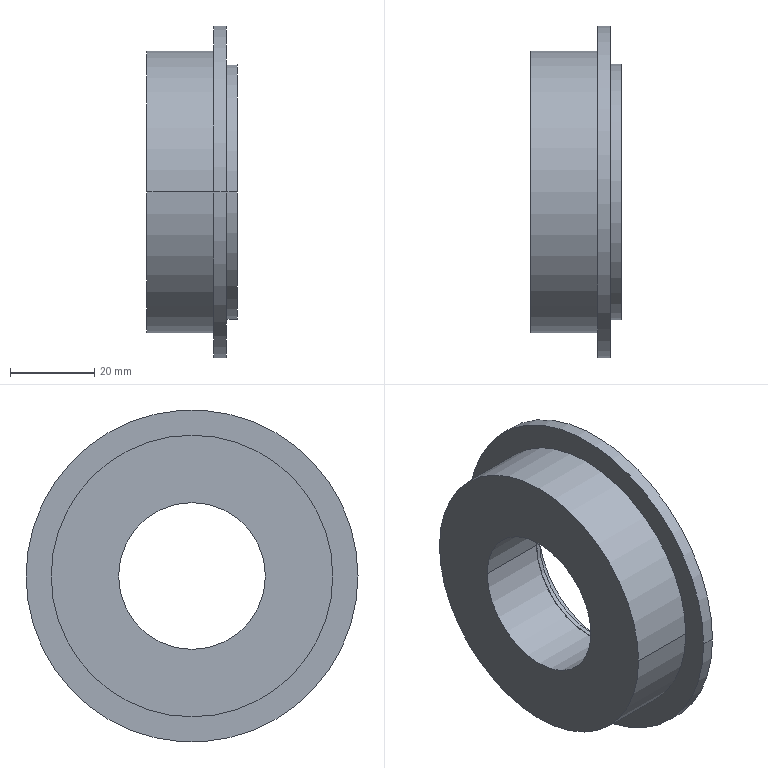Part | SolidWorks | features Revolution 1 | 4 solids | 39 faces | box 21.418 x 78.909 x 78.909 mm | volume 50880 mm3 | cylinder 26 | plane 13 | commonest cylinder face diameters 34.909 x4 40.909 x2 40.984 x2 42.979 x2 44.398 x2 50.004 x2
STEP:
#1=CARTESIAN_POINT('',(77.,20.455,0.));
#2=VERTEX_POINT('',#1);
#3=CARTESIAN_POINT('',(77.,-20.455,0.));
#4=VERTEX_POINT('',#3);
#5=CARTESIAN_POINT('',(77.,0.,0.));
#6=DIRECTION('',(1.,0.,0.));
#7=DIRECTION('',(0.,1.,0.));
#8=AXIS2_PLACEMENT_3D('',#5,#6,#7);
#9=CIRCLE('',#8,20.455);
#10=EDGE_CURVE('',#2,#4,#9,.T.);
#11=ORIENTED_EDGE('',*,*,#10,.T.);
#12=CARTESIAN_POINT('',(90.724,-20.455,0.));
#13=VERTEX_POINT('',#12);
#14=CARTESIAN_POINT('',(0.,-20.455,0.));
#15=DIRECTION('',(1.,0.,0.));
#16=VECTOR('',#15,1000.);
#17=LINE('',#14,#16);
#18=EDGE_CURVE('',#4,#13,#17,.T.);
#19=ORIENTED_EDGE('',*,*,#18,.T.);
#20=CARTESIAN_POINT('',(90.724,20.455,0.));
#21=VERTEX_POINT('',#20);
#22=CARTESIAN_POINT('',(90.724,0.,0.));
#23=DIRECTION('',(1.,0.,0.));
#24=DIRECTION('',(0.,1.,0.));
#25=AXIS2_PLACEMENT_3D('',#22,#23,#24);
#26=CIRCLE('',#25,20.455);
#27=EDGE_CURVE('',#21,#13,#26,.T.);
#28=ORIENTED_EDGE('',*,*,#27,.F.);
#29=CARTESIAN_POINT('',(0.,20.455,0.));
#30=DIRECTION('',(1.,0.,0.));
#31=VECTOR('',#30,1000.);
#32=LINE('',#29,#31);
#33=EDGE_CURVE('',#2,#21,#32,.T.);
#34=ORIENTED_EDGE('',*,*,#33,.F.);
#35=EDGE_LOOP('',(#11,#19,#28,#34));
#36=FACE_OUTER_BOUND('',#35,.T.);
#37=CARTESIAN_POINT('',(0.,0.,0.));
#38=DIRECTION('',(1.,0.,0.));
#39=DIRECTION('',(0.,1.,0.));
#40=AXIS2_PLACEMENT_3D('',#37,#38,#39);
#41=CYLINDRICAL_SURFACE('',#40,20.455);
#42=ADVANCED_FACE('',(#36),#41,.T.);
#43=CARTESIAN_POINT('',(74.143,-17.455,0.));
#44=VERTEX_POINT('',#43);
#45=CARTESIAN_POINT('',(74.143,17.455,0.));
#46=VERTEX_POINT('',#45);
#47=CARTESIAN_POINT('',(74.143,0.,0.));
#48=DIRECTION('',(1.,0.,0.));
#49=DIRECTION('',(0.,1.,0.));
#50=AXIS2_PLACEMENT_3D('',#47,#48,#49);
#51=CIRCLE('',#50,17.455);
#52=EDGE_CURVE('',#44,#46,#51,.T.);
#53=ORIENTED_EDGE('',*,*,#52,.F.);
#54=CARTESIAN_POINT('',(90.724,-17.455,0.));
#55=VERTEX_POINT('',#54);
#56=CARTESIAN_POINT('',(0.,-17.455,0.));
#57=DIRECTION('',(1.,0.,0.));
#58=VECTOR('',#57,1000.);
#59=LINE('',#56,#58);
#60=EDGE_CURVE('',#44,#55,#59,.T.);
#61=ORIENTED_EDGE('',*,*,#60,.T.);
#62=CARTESIAN_POINT('',(90.724,17.455,0.));
#63=VERTEX_POINT('',#62);
#64=CARTESIAN_POINT('',(90.724,0.,0.));
#65=DIRECTION('',(1.,0.,0.));
#66=DIRECTION('',(0.,1.,0.));
#67=AXIS2_PLACEMENT_3D('',#64,#65,#66);
#68=CIRCLE('',#67,17.455);
#69=EDGE_CURVE('',#55,#63,#68,.T.);
#70=ORIENTED_EDGE('',*,*,#69,.T.);
#71=CARTESIAN_POINT('',(0.,17.455,0.));
#72=DIRECTION('',(1.,0.,0.));
#73=VECTOR('',#72,1000.);
#74=LINE('',#71,#73);
#75=EDGE_CURVE('',#46,#63,#74,.T.);
#76=ORIENTED_EDGE('',*,*,#75,.F.);
#77=EDGE_LOOP('',(#53,#61,#70,#76));
#78=FACE_OUTER_BOUND('',#77,.T.);
#79=CARTESIAN_POINT('',(0.,0.,0.));
#80=DIRECTION('',(1.,0.,0.));
#81=DIRECTION('',(0.,1.,0.));
#82=AXIS2_PLACEMENT_3D('',#79,#80,#81);
#83=CYLINDRICAL_SURFACE('',#82,17.455);
#84=ADVANCED_FACE('',(#78),#83,.F.);
#85=CARTESIAN_POINT('',(74.143,33.455,0.));
#86=VERTEX_POINT('',#85);
#87=CARTESIAN_POINT('',(74.143,-33.455,0.));
#88=VERTEX_POINT('',#87);
#89=CARTESIAN_POINT('',(74.143,0.,0.));
#90=DIRECTION('',(1.,0.,0.));
#91=DIRECTION('',(0.,1.,0.));
#92=AXIS2_PLACEMENT_3D('',#89,#90,#91);
#93=CIRCLE('',#92,33.455);
#94=EDGE_CURVE('',#86,#88,#93,.T.);
#95=ORIENTED_EDGE('',*,*,#94,.T.);
#96=CARTESIAN_POINT('',(90.,-33.455,0.));
#97=VERTEX_POINT('',#96);
#98=CARTESIAN_POINT('',(0.,-33.455,0.));
#99=DIRECTION('',(1.,0.,0.));
#100=VECTOR('',#99,1000.);
#101=LINE('',#98,#100);
#102=EDGE_CURVE('',#88,#97,#101,.T.);
#103=ORIENTED_EDGE('',*,*,#102,.T.);
#104=CARTESIAN_POINT('',(90.,33.455,0.));
#105=VERTEX_POINT('',#104);
#106=CARTESIAN_POINT('',(90.,0.,0.));
#107=DIRECTION('',(1.,0.,0.));
#108=DIRECTION('',(0.,1.,0.));
#109=AXIS2_PLACEMENT_3D('',#106,#107,#108);
#110=CIRCLE('',#109,33.455);
#111=EDGE_CURVE('',#105,#97,#110,.T.);
#112=ORIENTED_EDGE('',*,*,#111,.F.);
#113=CARTESIAN_POINT('',(0.,33.455,0.));
#114=DIRECTION('',(1.,0.,0.));
#115=VECTOR('',#114,1000.);
#116=LINE('',#113,#115);
#117=EDGE_CURVE('',#86,#105,#116,.T.);
#118=ORIENTED_EDGE('',*,*,#117,.F.);
#119=EDGE_LOOP('',(#95,#103,#112,#118));
#120=FACE_OUTER_BOUND('',#119,.T.);
#121=CARTESIAN_POINT('',(0.,0.,0.));
#122=DIRECTION('',(1.,0.,0.));
#123=DIRECTION('',(0.,1.,0.));
#124=AXIS2_PLACEMENT_3D('',#121,#122,#123);
#125=CYLINDRICAL_SURFACE('',#124,33.455);
#126=ADVANCED_FACE('',(#120),#125,.T.);
#127=CARTESIAN_POINT('',(90.,39.455,0.));
#128=VERTEX_POINT('',#127);
#129=CARTESIAN_POINT('',(90.,-39.455,0.));
#130=VERTEX_POINT('',#129);
#131=CARTESIAN_POINT('',(90.,0.,0.));
#132=DIRECTION('',(1.,0.,0.));
#133=DIRECTION('',(0.,1.,0.));
#134=AXIS2_PLACEMENT_3D('',#131,#132,#133);
#135=CIRCLE('',#134,39.455);
#136=EDGE_CURVE('',#128,#130,#135,.T.);
#137=ORIENTED_EDGE('',*,*,#136,.T.);
#138=CARTESIAN_POINT('',(93.,-39.455,0.));
#139=VERTEX_POINT('',#138);
#140=CARTESIAN_POINT('',(0.,-39.455,0.));
#141=DIRECTION('',(1.,0.,0.));
#142=VECTOR('',#141,1000.);
#143=LINE('',#140,#142);
#144=EDGE_CURVE('',#130,#139,#143,.T.);
#145=ORIENTED_EDGE('',*,*,#144,.T.);
#146=CARTESIAN_POINT('',(93.,39.455,0.));
#147=VERTEX_POINT('',#146);
#148=CARTESIAN_POINT('',(93.,0.,0.));
#149=DIRECTION('',(1.,0.,0.));
#150=DIRECTION('',(0.,1.,0.));
#151=AXIS2_PLACEMENT_3D('',#148,#149,#150);
#152=CIRCLE('',#151,39.455);
#153=EDGE_CURVE('',#147,#139,#152,.T.);
#154=ORIENTED_EDGE('',*,*,#153,.F.);
#155=CARTESIAN_POINT('',(0.,39.455,0.));
#156=DIRECTION('',(1.,0.,0.));
#157=VECTOR('',#156,1000.);
#158=LINE('',#155,#157);
#159=EDGE_CURVE('',#128,#147,#158,.T.);
#160=ORIENTED_EDGE('',*,*,#159,.F.);
#161=EDGE_LOOP('',(#137,#145,#154,#160));
#162=FACE_OUTER_BOUND('',#161,.T.);
#163=CARTESIAN_POINT('',(0.,0.,0.));
#164=DIRECTION('',(1.,0.,0.));
#165=DIRECTION('',(0.,1.,0.));
#166=AXIS2_PLACEMENT_3D('',#163,#164,#165);
#167=CYLINDRICAL_SURFACE('',#166,39.455);
#168=ADVANCED_FACE('',(#162),#167,.T.);
#169=CARTESIAN_POINT('',(77.,-30.955,0.));
#170=VERTEX_POINT('',#169);
#171=CARTESIAN_POINT('',(77.,30.955,0.));
#172=VERTEX_POINT('',#171);
#173=CARTESIAN_POINT('',(77.,0.,0.));
#174=DIRECTION('',(1.,0.,0.));
#175=DIRECTION('',(0.,1.,0.));
#176=AXIS2_PLACEMENT_3D('',#173,#174,#175);
#177=CIRCLE('',#176,30.955);
#178=EDGE_CURVE('',#170,#172,#177,.T.);
#179=ORIENTED_EDGE('',*,*,#178,.F.);
#180=CARTESIAN_POINT('',(93.,-30.955,0.));
#181=VERTEX_POINT('',#180);
#182=CARTESIAN_POINT('',(0.,-30.955,0.));
#183=DIRECTION('',(1.,0.,0.));
#184=VECTOR('',#183,1000.);
#185=LINE('',#182,#184);
#186=EDGE_CURVE('',#170,#181,#185,.T.);
#187=ORIENTED_EDGE('',*,*,#186,.T.);
#188=CARTESIAN_POINT('',(93.,30.955,0.));
#189=VERTEX_POINT('',#188);
#190=CARTESIAN_POINT('',(93.,0.,0.));
#191=DIRECTION('',(1.,0.,0.));
#192=DIRECTION('',(0.,1.,0.));
#193=AXIS2_PLACEMENT_3D('',#190,#191,#192);
#194=CIRCLE('',#193,30.955);
#195=EDGE_CURVE('',#181,#189,#194,.T.);
#196=ORIENTED_EDGE('',*,*,#195,.T.);
#197=CARTESIAN_POINT('',(0.,30.955,0.));
#198=DIRECTION('',(1.,0.,0.));
#199=VECTOR('',#198,1000.);
#200=LINE('',#197,#199);
#201=EDGE_CURVE('',#172,#189,#200,.T.);
#202=ORIENTED_EDGE('',*,*,#201,.F.);
#203=EDGE_LOOP('',(#179,#187,#196,#202));
#204=FACE_OUTER_BOUND('',#203,.T.);
#205=CARTESIAN_POINT('',(0.,0.,0.));
#206=DIRECTION('',(1.,0.,0.));
#207=DIRECTION('',(0.,1.,0.));
#208=AXIS2_PLACEMENT_3D('',#205,#206,#207);
#209=CYLINDRICAL_SURFACE('',#208,30.955);
#210=ADVANCED_FACE('',(#204),#209,.F.);
#211=ORIENTED_EDGE('',*,*,#186,.F.);
#212=CARTESIAN_POINT('',(77.,0.,0.));
#213=DIRECTION('',(1.,0.,0.));
#214=DIRECTION('',(0.,1.,0.));
#215=AXIS2_PLACEMENT_3D('',#212,#213,#214);
#216=CIRCLE('',#215,30.955);
#217=EDGE_CURVE('',#172,#170,#216,.T.);
#218=ORIENTED_EDGE('',*,*,#217,.F.);
#219=ORIENTED_EDGE('',*,*,#201,.T.);
#220=CARTESIAN_POINT('',(93.,0.,0.));
#221=DIRECTION('',(1.,0.,0.));
#222=DIRECTION('',(0.,1.,0.));
#223=AXIS2_PLACEMENT_3D('',#220,#221,#222);
#224=CIRCLE('',#223,30.955);
#225=EDGE_CURVE('',#189,#181,#224,.T.);
#226=ORIENTED_EDGE('',*,*,#225,.T.);
#227=EDGE_LOOP('',(#211,#218,#219,#226));
#228=FACE_OUTER_BOUND('',#227,.T.);
#229=CARTESIAN_POINT('',(0.,0.,0.));
#230=DIRECTION('',(1.,0.,0.));
#231=DIRECTION('',(0.,1.,0.));
#232=AXIS2_PLACEMENT_3D('',#229,#230,#231);
#233=CYLINDRICAL_SURFACE('',#232,30.955);
#234=ADVANCED_FACE('',(#228),#233,.F.);
#235=ORIENTED_EDGE('',*,*,#153,.T.);
#236=CARTESIAN_POINT('',(93.,0.,0.));
#237=DIRECTION('',(1.,0.,0.));
#238=DIRECTION('',(0.,1.,0.));
#239=AXIS2_PLACEMENT_3D('',#236,#237,#238);
#240=CIRCLE('',#239,39.455);
#241=EDGE_CURVE('',#139,#147,#240,.T.);
#242=ORIENTED_EDGE('',*,*,#241,.T.);
#243=EDGE_LOOP('',(#235,#242));
#244=FACE_OUTER_BOUND('',#243,.T.);
#245=ORIENTED_EDGE('',*,*,#225,.F.);
#246=ORIENTED_EDGE('',*,*,#195,.F.);
#247=EDGE_LOOP('',(#245,#246));
#248=FACE_BOUND('',#247,.T.);
#249=CARTESIAN_POINT('',(93.,0.,0.));
#250=DIRECTION('',(1.,0.,0.));
#251=DIRECTION('',(0.,1.,0.));
#252=AXIS2_PLACEMENT_3D('',#249,#250,#251);
#253=PLANE('',#252);
#254=ADVANCED_FACE('',(#244,#248),#253,.T.);
#255=ORIENTED_EDGE('',*,*,#144,.F.);
#256=CARTESIAN_POINT('',(90.,0.,0.));
#257=DIRECTION('',(1.,0.,0.));
#258=DIRECTION('',(0.,1.,0.));
#259=AXIS2_PLACEMENT_3D('',#256,#257,#258);
#260=CIRCLE('',#259,39.455);
#261=EDGE_CURVE('',#130,#128,#260,.T.);
#262=ORIENTED_EDGE('',*,*,#261,.T.);
#263=ORIENTED_EDGE('',*,*,#159,.T.);
#264=ORIENTED_EDGE('',*,*,#241,.F.);
#265=EDGE_LOOP('',(#255,#262,#263,#264));
#266=FACE_OUTER_BOUND('',#265,.T.);
#267=CARTESIAN_POINT('',(0.,0.,0.));
#268=DIRECTION('',(1.,0.,0.));
#269=DIRECTION('',(0.,1.,0.));
#270=AXIS2_PLACEMENT_3D('',#267,#268,#269);
#271=CYLINDRICAL_SURFACE('',#270,39.455);
#272=ADVANCED_FACE('',(#266),#271,.T.);
#273=ORIENTED_EDGE('',*,*,#136,.F.);
#274=ORIENTED_EDGE('',*,*,#261,.F.);
#275=EDGE_LOOP('',(#273,#274));
#276=FACE_OUTER_BOUND('',#275,.T.);
#277=ORIENTED_EDGE('',*,*,#111,.T.);
#278=CARTESIAN_POINT('',(90.,0.,0.));
#279=DIRECTION('',(1.,0.,0.));
#280=DIRECTION('',(0.,1.,0.));
#281=AXIS2_PLACEMENT_3D('',#278,#279,#280);
#282=CIRCLE('',#281,33.455);
#283=EDGE_CURVE('',#97,#105,#282,.T.);
#284=ORIENTED_EDGE('',*,*,#283,.T.);
#285=EDGE_LOOP('',(#277,#284));
#286=FACE_BOUND('',#285,.T.);
#287=CARTESIAN_POINT('',(90.,0.,0.));
#288=DIRECTION('',(1.,0.,0.));
#289=DIRECTION('',(0.,1.,0.));
#290=AXIS2_PLACEMENT_3D('',#287,#288,#289);
#291=PLANE('',#290);
#292=ADVANCED_FACE('',(#276,#286),#291,.F.);
#293=ORIENTED_EDGE('',*,*,#102,.F.);
#294=CARTESIAN_POINT('',(74.143,0.,0.));
#295=DIRECTION('',(1.,0.,0.));
#296=DIRECTION('',(0.,1.,0.));
#297=AXIS2_PLACEMENT_3D('',#294,#295,#296);
#298=CIRCLE('',#297,33.455);
#299=EDGE_CURVE('',#88,#86,#298,.T.);
#300=ORIENTED_EDGE('',*,*,#299,.T.);
#301=ORIENTED_EDGE('',*,*,#117,.T.);
#302=ORIENTED_EDGE('',*,*,#283,.F.);
#303=EDGE_LOOP('',(#293,#300,#301,#302));
#304=FACE_OUTER_BOUND('',#303,.T.);
#305=CARTESIAN_POINT('',(0.,0.,0.));
#306=DIRECTION('',(1.,0.,0.));
#307=DIRECTION('',(0.,1.,0.));
#308=AXIS2_PLACEMENT_3D('',#305,#306,#307);
#309=CYLINDRICAL_SURFACE('',#308,33.455);
#310=ADVANCED_FACE('',(#304),#309,.T.);
#311=CARTESIAN_POINT('',(74.143,0.,0.));
#312=DIRECTION('',(1.,0.,0.));
#313=DIRECTION('',(0.,1.,0.));
#314=AXIS2_PLACEMENT_3D('',#311,#312,#313);
#315=CIRCLE('',#314,17.455);
#316=EDGE_CURVE('',#46,#44,#315,.T.);
#317=ORIENTED_EDGE('',*,*,#316,.T.);
#318=ORIENTED_EDGE('',*,*,#52,.T.);
#319=EDGE_LOOP('',(#317,#318));
#320=FACE_BOUND('',#319,.T.);
#321=ORIENTED_EDGE('',*,*,#94,.F.);
#322=ORIENTED_EDGE('',*,*,#299,.F.);
#323=EDGE_LOOP('',(#321,#322));
#324=FACE_OUTER_BOUND('',#323,.T.);
#325=CARTESIAN_POINT('',(74.143,0.,0.));
#326=DIRECTION('',(-1.,0.,0.));
#327=DIRECTION('',(0.,-1.,0.));
#328=AXIS2_PLACEMENT_3D('',#325,#326,#327);
#329=PLANE('',#328);
#330=ADVANCED_FACE('',(#320,#324),#329,.T.);
#331=ORIENTED_EDGE('',*,*,#60,.F.);
#332=ORIENTED_EDGE('',*,*,#316,.F.);
#333=ORIENTED_EDGE('',*,*,#75,.T.);
#334=CARTESIAN_POINT('',(90.724,0.,0.));
#335=DIRECTION('',(1.,0.,0.));
#336=DIRECTION('',(0.,1.,0.));
#337=AXIS2_PLACEMENT_3D('',#334,#335,#336);
#338=CIRCLE('',#337,17.455);
#339=EDGE_CURVE('',#63,#55,#338,.T.);
#340=ORIENTED_EDGE('',*,*,#339,.T.);
#341=EDGE_LOOP('',(#331,#332,#333,#340));
#342=FACE_OUTER_BOUND('',#341,.T.);
#343=CARTESIAN_POINT('',(0.,0.,0.));
#344=DIRECTION('',(1.,0.,0.));
#345=DIRECTION('',(0.,1.,0.));
#346=AXIS2_PLACEMENT_3D('',#343,#344,#345);
#347=CYLINDRICAL_SURFACE('',#346,17.455);
#348=ADVANCED_FACE('',(#342),#347,.F.);
#349=ORIENTED_EDGE('',*,*,#27,.T.);
#350=CARTESIAN_POINT('',(90.724,0.,0.));
#351=DIRECTION('',(1.,0.,0.));
#352=DIRECTION('',(0.,1.,0.));
#353=AXIS2_PLACEMENT_3D('',#350,#351,#352);
#354=CIRCLE('',#353,20.455);
#355=EDGE_CURVE('',#13,#21,#354,.T.);
#356=ORIENTED_EDGE('',*,*,#355,.T.);
#357=EDGE_LOOP('',(#349,#356));
#358=FACE_OUTER_BOUND('',#357,.T.);
#359=ORIENTED_EDGE('',*,*,#339,.F.);
#360=ORIENTED_EDGE('',*,*,#69,.F.);
#361=EDGE_LOOP('',(#359,#360));
#362=FACE_BOUND('',#361,.T.);
#363=CARTESIAN_POINT('',(90.724,0.,0.));
#364=DIRECTION('',(1.,0.,0.));
#365=DIRECTION('',(0.,1.,0.));
#366=AXIS2_PLACEMENT_3D('',#363,#364,#365);
#367=PLANE('',#366);
#368=ADVANCED_FACE('',(#358,#362),#367,.T.);
#369=ORIENTED_EDGE('',*,*,#18,.F.);
#370=CARTESIAN_POINT('',(77.,0.,0.));
#371=DIRECTION('',(1.,0.,0.));
#372=DIRECTION('',(0.,1.,0.));
#373=AXIS2_PLACEMENT_3D('',#370,#371,#372);
#374=CIRCLE('',#373,20.455);
#375=EDGE_CURVE('',#4,#2,#374,.T.);
#376=ORIENTED_EDGE('',*,*,#375,.T.);
#377=ORIENTED_EDGE('',*,*,#33,.T.);
#378=ORIENTED_EDGE('',*,*,#355,.F.);
#379=EDGE_LOOP('',(#369,#376,#377,#378));
#380=FACE_OUTER_BOUND('',#379,.T.);
#381=CARTESIAN_POINT('',(0.,0.,0.));
#382=DIRECTION('',(1.,0.,0.));
#383=DIRECTION('',(0.,1.,0.));
#384=AXIS2_PLACEMENT_3D('',#381,#382,#383);
#385=CYLINDRICAL_SURFACE('',#384,20.455);
#386=ADVANCED_FACE('',(#380),#385,.T.);
#387=ORIENTED_EDGE('',*,*,#217,.T.);
#388=ORIENTED_EDGE('',*,*,#178,.T.);
#389=EDGE_LOOP('',(#387,#388));
#390=FACE_OUTER_BOUND('',#389,.T.);
#391=ORIENTED_EDGE('',*,*,#10,.F.);
#392=ORIENTED_EDGE('',*,*,#375,.F.);
#393=EDGE_LOOP('',(#391,#392));
#394=FACE_BOUND('',#393,.T.);
#395=CARTESIAN_POINT('',(77.,0.,0.));
#396=DIRECTION('',(1.,0.,0.));
#397=DIRECTION('',(0.,1.,0.));
#398=AXIS2_PLACEMENT_3D('',#395,#396,#397);
#399=PLANE('',#398);
#400=ADVANCED_FACE('',(#390,#394),#399,.T.);
#401=CLOSED_SHELL('',(#42,#84,#126,#168,#210,#234,#254,#272,#292,#310,#330,#348,#368,#386,#400));
#402=MANIFOLD_SOLID_BREP('',#401);
#403=CARTESIAN_POINT('',(90.724,-25.002,0.));
#404=VERTEX_POINT('',#403);
#405=CARTESIAN_POINT('',(90.724,25.002,0.));
#406=VERTEX_POINT('',#405);
#407=CARTESIAN_POINT('',(90.724,0.,0.));
#408=DIRECTION('',(1.,0.,0.));
#409=DIRECTION('',(0.,1.,0.));
#410=AXIS2_PLACEMENT_3D('',#407,#408,#409);
#411=CIRCLE('',#410,25.002);
#412=EDGE_CURVE('',#404,#406,#411,.T.);
#413=ORIENTED_EDGE('',*,*,#412,.F.);
#414=CARTESIAN_POINT('',(93.034,-25.002,0.));
#415=VERTEX_POINT('',#414);
#416=CARTESIAN_POINT('',(0.,-25.002,0.));
#417=DIRECTION('',(1.,0.,0.));
#418=VECTOR('',#417,1000.);
#419=LINE('',#416,#418);
#420=EDGE_CURVE('',#404,#415,#419,.T.);
#421=ORIENTED_EDGE('',*,*,#420,.T.);
#422=CARTESIAN_POINT('',(93.034,25.002,0.));
#423=VERTEX_POINT('',#422);
#424=CARTESIAN_POINT('',(93.034,0.,0.));
#425=DIRECTION('',(1.,0.,0.));
#426=DIRECTION('',(0.,1.,0.));
#427=AXIS2_PLACEMENT_3D('',#424,#425,#426);
#428=CIRCLE('',#427,25.002);
#429=EDGE_CURVE('',#415,#423,#428,.T.);
#430=ORIENTED_EDGE('',*,*,#429,.T.);
#431=CARTESIAN_POINT('',(0.,25.002,0.));
#432=DIRECTION('',(1.,0.,0.));
#433=VECTOR('',#432,1000.);
#434=LINE('',#431,#433);
#435=EDGE_CURVE('',#406,#423,#434,.T.);
#436=ORIENTED_EDGE('',*,*,#435,.F.);
#437=EDGE_LOOP('',(#413,#421,#430,#436));
#438=FACE_OUTER_BOUND('',#437,.T.);
#439=CARTESIAN_POINT('',(0.,0.,0.));
#440=DIRECTION('',(1.,0.,0.));
#441=DIRECTION('',(0.,1.,0.));
#442=AXIS2_PLACEMENT_3D('',#439,#440,#441);
#443=CYLINDRICAL_SURFACE('',#442,25.002);
#444=ADVANCED_FACE('',(#438),#443,.F.);
#445=CARTESIAN_POINT('',(77.848,-26.574,0.));
#446=VERTEX_POINT('',#445);
#447=CARTESIAN_POINT('',(77.848,26.574,0.));
#448=VERTEX_POINT('',#447);
#449=CARTESIAN_POINT('',(77.848,0.,0.));
#450=DIRECTION('',(1.,0.,0.));
#451=DIRECTION('',(0.,1.,0.));
#452=AXIS2_PLACEMENT_3D('',#449,#450,#451);
#453=CIRCLE('',#452,26.574);
#454=EDGE_CURVE('',#446,#448,#453,.T.);
#455=ORIENTED_EDGE('',*,*,#454,.F.);
#456=CARTESIAN_POINT('',(90.724,-26.574,0.));
#457=VERTEX_POINT('',#456);
#458=CARTESIAN_POINT('',(0.,-26.574,0.));
#459=DIRECTION('',(1.,0.,0.));
#460=VECTOR('',#459,1000.);
#461=LINE('',#458,#460);
#462=EDGE_CURVE('',#446,#457,#461,.T.);
#463=ORIENTED_EDGE('',*,*,#462,.T.);
#464=CARTESIAN_POINT('',(90.724,26.574,0.));
#465=VERTEX_POINT('',#464);
#466=CARTESIAN_POINT('',(90.724,0.,0.));
#467=DIRECTION('',(1.,0.,0.));
#468=DIRECTION('',(0.,1.,0.));
#469=AXIS2_PLACEMENT_3D('',#466,#467,#468);
#470=CIRCLE('',#469,26.574);
#471=EDGE_CURVE('',#457,#465,#470,.T.);
#472=ORIENTED_EDGE('',*,*,#471,.T.);
#473=CARTESIAN_POINT('',(0.,26.574,0.));
#474=DIRECTION('',(1.,0.,0.));
#475=VECTOR('',#474,1000.);
#476=LINE('',#473,#475);
#477=EDGE_CURVE('',#448,#465,#476,.T.);
#478=ORIENTED_EDGE('',*,*,#477,.F.);
#479=EDGE_LOOP('',(#455,#463,#472,#478));
#480=FACE_OUTER_BOUND('',#479,.T.);
#481=CARTESIAN_POINT('',(0.,0.,0.));
#482=DIRECTION('',(1.,0.,0.));
#483=DIRECTION('',(0.,1.,0.));
#484=AXIS2_PLACEMENT_3D('',#481,#482,#483);
#485=CYLINDRICAL_SURFACE('',#484,26.574);
#486=ADVANCED_FACE('',(#480),#485,.F.);
#487=CARTESIAN_POINT('',(77.848,30.355,0.));
#488=VERTEX_POINT('',#487);
#489=CARTESIAN_POINT('',(77.848,-30.355,0.));
#490=VERTEX_POINT('',#489);
#491=CARTESIAN_POINT('',(77.848,0.,0.));
#492=DIRECTION('',(1.,0.,0.));
#493=DIRECTION('',(0.,1.,0.));
#494=AXIS2_PLACEMENT_3D('',#491,#492,#493);
#495=CIRCLE('',#494,30.355);
#496=EDGE_CURVE('',#488,#490,#495,.T.);
#497=ORIENTED_EDGE('',*,*,#496,.T.);
#498=CARTESIAN_POINT('',(95.561,-30.355,0.));
#499=VERTEX_POINT('',#498);
#500=CARTESIAN_POINT('',(0.,-30.355,0.));
#501=DIRECTION('',(1.,0.,0.));
#502=VECTOR('',#501,1000.);
#503=LINE('',#500,#502);
#504=EDGE_CURVE('',#490,#499,#503,.T.);
#505=ORIENTED_EDGE('',*,*,#504,.T.);
#506=CARTESIAN_POINT('',(95.561,30.355,0.));
#507=VERTEX_POINT('',#506);
#508=CARTESIAN_POINT('',(95.561,0.,0.));
#509=DIRECTION('',(1.,0.,0.));
#510=DIRECTION('',(0.,1.,0.));
#511=AXIS2_PLACEMENT_3D('',#508,#509,#510);
#512=CIRCLE('',#511,30.355);
#513=EDGE_CURVE('',#507,#499,#512,.T.);
#514=ORIENTED_EDGE('',*,*,#513,.F.);
#515=CARTESIAN_POINT('',(0.,30.355,0.));
#516=DIRECTION('',(1.,0.,0.));
#517=VECTOR('',#516,1000.);
#518=LINE('',#515,#517);
#519=EDGE_CURVE('',#488,#507,#518,.T.);
#520=ORIENTED_EDGE('',*,*,#519,.F.);
#521=EDGE_LOOP('',(#497,#505,#514,#520));
#522=FACE_OUTER_BOUND('',#521,.T.);
#523=CARTESIAN_POINT('',(0.,0.,0.));
#524=DIRECTION('',(1.,0.,0.));
#525=DIRECTION('',(0.,1.,0.));
#526=AXIS2_PLACEMENT_3D('',#523,#524,#525);
#527=CYLINDRICAL_SURFACE('',#526,30.355);
#528=ADVANCED_FACE('',(#522),#527,.T.);
#529=CARTESIAN_POINT('',(93.034,-21.49,0.));
#530=VERTEX_POINT('',#529);
#531=CARTESIAN_POINT('',(93.034,21.49,0.));
#532=VERTEX_POINT('',#531);
#533=CARTESIAN_POINT('',(93.034,0.,0.));
#534=DIRECTION('',(1.,0.,0.));
#535=DIRECTION('',(0.,1.,0.));
#536=AXIS2_PLACEMENT_3D('',#533,#534,#535);
#537=CIRCLE('',#536,21.49);
#538=EDGE_CURVE('',#530,#532,#537,.T.);
#539=ORIENTED_EDGE('',*,*,#538,.F.);
#540=CARTESIAN_POINT('',(95.561,-21.49,0.));
#541=VERTEX_POINT('',#540);
#542=CARTESIAN_POINT('',(0.,-21.49,0.));
#543=DIRECTION('',(1.,0.,0.));
#544=VECTOR('',#543,1000.);
#545=LINE('',#542,#544);
#546=EDGE_CURVE('',#530,#541,#545,.T.);
#547=ORIENTED_EDGE('',*,*,#546,.T.);
#548=CARTESIAN_POINT('',(95.561,21.49,0.));
#549=VERTEX_POINT('',#548);
#550=CARTESIAN_POINT('',(95.561,0.,0.));
#551=DIRECTION('',(1.,0.,0.));
#552=DIRECTION('',(0.,1.,0.));
#553=AXIS2_PLACEMENT_3D('',#550,#551,#552);
#554=CIRCLE('',#553,21.49);
#555=EDGE_CURVE('',#541,#549,#554,.T.);
#556=ORIENTED_EDGE('',*,*,#555,.T.);
#557=CARTESIAN_POINT('',(0.,21.49,0.));
#558=DIRECTION('',(1.,0.,0.));
#559=VECTOR('',#558,1000.);
#560=LINE('',#557,#559);
#561=EDGE_CURVE('',#532,#549,#560,.T.);
#562=ORIENTED_EDGE('',*,*,#561,.F.);
#563=EDGE_LOOP('',(#539,#547,#556,#562));
#564=FACE_OUTER_BOUND('',#563,.T.);
#565=CARTESIAN_POINT('',(0.,0.,0.));
#566=DIRECTION('',(1.,0.,0.));
#567=DIRECTION('',(0.,1.,0.));
#568=AXIS2_PLACEMENT_3D('',#565,#566,#567);
#569=CYLINDRICAL_SURFACE('',#568,21.49);
#570=ADVANCED_FACE('',(#564),#569,.F.);
#571=CARTESIAN_POINT('',(93.034,0.,0.));
#572=DIRECTION('',(1.,0.,0.));
#573=DIRECTION('',(0.,1.,0.));
#574=AXIS2_PLACEMENT_3D('',#571,#572,#573);
#575=CIRCLE('',#574,25.002);
#576=EDGE_CURVE('',#423,#415,#575,.T.);
#577=ORIENTED_EDGE('',*,*,#576,.F.);
#578=ORIENTED_EDGE('',*,*,#429,.F.);
#579=EDGE_LOOP('',(#577,#578));
#580=FACE_OUTER_BOUND('',#579,.T.);
#581=CARTESIAN_POINT('',(93.034,0.,0.));
#582=DIRECTION('',(1.,0.,0.));
#583=DIRECTION('',(0.,1.,0.));
#584=AXIS2_PLACEMENT_3D('',#581,#582,#583);
#585=CIRCLE('',#584,21.49);
#586=EDGE_CURVE('',#532,#530,#585,.T.);
#587=ORIENTED_EDGE('',*,*,#586,.T.);
#588=ORIENTED_EDGE('',*,*,#538,.T.);
#589=EDGE_LOOP('',(#587,#588));
#590=FACE_BOUND('',#589,.T.);
#591=CARTESIAN_POINT('',(93.034,0.,0.));
#592=DIRECTION('',(1.,0.,0.));
#593=DIRECTION('',(0.,1.,0.));
#594=AXIS2_PLACEMENT_3D('',#591,#592,#593);
#595=PLANE('',#594);
#596=ADVANCED_FACE('',(#580,#590),#595,.F.);
#597=ORIENTED_EDGE('',*,*,#546,.F.);
#598=ORIENTED_EDGE('',*,*,#586,.F.);
#599=ORIENTED_EDGE('',*,*,#561,.T.);
#600=CARTESIAN_POINT('',(95.561,0.,0.));
#601=DIRECTION('',(1.,0.,0.));
#602=DIRECTION('',(0.,1.,0.));
#603=AXIS2_PLACEMENT_3D('',#600,#601,#602);
#604=CIRCLE('',#603,21.49);
#605=EDGE_CURVE('',#549,#541,#604,.T.);
#606=ORIENTED_EDGE('',*,*,#605,.T.);
#607=EDGE_LOOP('',(#597,#598,#599,#606));
#608=FACE_OUTER_BOUND('',#607,.T.);
#609=CARTESIAN_POINT('',(0.,0.,0.));
#610=DIRECTION('',(1.,0.,0.));
#611=DIRECTION('',(0.,1.,0.));
#612=AXIS2_PLACEMENT_3D('',#609,#610,#611);
#613=CYLINDRICAL_SURFACE('',#612,21.49);
#614=ADVANCED_FACE('',(#608),#613,.F.);
#615=ORIENTED_EDGE('',*,*,#605,.F.);
#616=ORIENTED_EDGE('',*,*,#555,.F.);
#617=EDGE_LOOP('',(#615,#616));
#618=FACE_BOUND('',#617,.T.);
#619=ORIENTED_EDGE('',*,*,#513,.T.);
#620=CARTESIAN_POINT('',(95.561,0.,0.));
#621=DIRECTION('',(1.,0.,0.));
#622=DIRECTION('',(0.,1.,0.));
#623=AXIS2_PLACEMENT_3D('',#620,#621,#622);
#624=CIRCLE('',#623,30.355);
#625=EDGE_CURVE('',#499,#507,#624,.T.);
#626=ORIENTED_EDGE('',*,*,#625,.T.);
#627=EDGE_LOOP('',(#619,#626));
#628=FACE_OUTER_BOUND('',#627,.T.);
#629=CARTESIAN_POINT('',(95.561,0.,0.));
#630=DIRECTION('',(-1.,0.,0.));
#631=DIRECTION('',(0.,-1.,0.));
#632=AXIS2_PLACEMENT_3D('',#629,#630,#631);
#633=PLANE('',#632);
#634=ADVANCED_FACE('',(#618,#628),#633,.F.);
#635=ORIENTED_EDGE('',*,*,#504,.F.);
#636=CARTESIAN_POINT('',(77.848,0.,0.));
#637=DIRECTION('',(1.,0.,0.));
#638=DIRECTION('',(0.,1.,0.));
#639=AXIS2_PLACEMENT_3D('',#636,#637,#638);
#640=CIRCLE('',#639,30.355);
#641=EDGE_CURVE('',#490,#488,#640,.T.);
#642=ORIENTED_EDGE('',*,*,#641,.T.);
#643=ORIENTED_EDGE('',*,*,#519,.T.);
#644=ORIENTED_EDGE('',*,*,#625,.F.);
#645=EDGE_LOOP('',(#635,#642,#643,#644));
#646=FACE_OUTER_BOUND('',#645,.T.);
#647=CARTESIAN_POINT('',(0.,0.,0.));
#648=DIRECTION('',(1.,0.,0.));
#649=DIRECTION('',(0.,1.,0.));
#650=AXIS2_PLACEMENT_3D('',#647,#648,#649);
#651=CYLINDRICAL_SURFACE('',#650,30.355);
#652=ADVANCED_FACE('',(#646),#651,.T.);
#653=ORIENTED_EDGE('',*,*,#496,.F.);
#654=ORIENTED_EDGE('',*,*,#641,.F.);
#655=EDGE_LOOP('',(#653,#654));
#656=FACE_OUTER_BOUND('',#655,.T.);
#657=CARTESIAN_POINT('',(77.848,0.,0.));
#658=DIRECTION('',(1.,0.,0.));
#659=DIRECTION('',(0.,1.,0.));
#660=AXIS2_PLACEMENT_3D('',#657,#658,#659);
#661=CIRCLE('',#660,26.574);
#662=EDGE_CURVE('',#448,#446,#661,.T.);
#663=ORIENTED_EDGE('',*,*,#662,.T.);
#664=ORIENTED_EDGE('',*,*,#454,.T.);
#665=EDGE_LOOP('',(#663,#664));
#666=FACE_BOUND('',#665,.T.);
#667=CARTESIAN_POINT('',(77.848,0.,0.));
#668=DIRECTION('',(1.,0.,0.));
#669=DIRECTION('',(0.,1.,0.));
#670=AXIS2_PLACEMENT_3D('',#667,#668,#669);
#671=PLANE('',#670);
#672=ADVANCED_FACE('',(#656,#666),#671,.F.);
#673=ORIENTED_EDGE('',*,*,#462,.F.);
#674=ORIENTED_EDGE('',*,*,#662,.F.);
#675=ORIENTED_EDGE('',*,*,#477,.T.);
#676=CARTESIAN_POINT('',(90.724,0.,0.));
#677=DIRECTION('',(1.,0.,0.));
#678=DIRECTION('',(0.,1.,0.));
#679=AXIS2_PLACEMENT_3D('',#676,#677,#678);
#680=CIRCLE('',#679,26.574);
#681=EDGE_CURVE('',#465,#457,#680,.T.);
#682=ORIENTED_EDGE('',*,*,#681,.T.);
#683=EDGE_LOOP('',(#673,#674,#675,#682));
#684=FACE_OUTER_BOUND('',#683,.T.);
#685=CARTESIAN_POINT('',(0.,0.,0.));
#686=DIRECTION('',(1.,0.,0.));
#687=DIRECTION('',(0.,1.,0.));
#688=AXIS2_PLACEMENT_3D('',#685,#686,#687);
#689=CYLINDRICAL_SURFACE('',#688,26.574);
#690=ADVANCED_FACE('',(#684),#689,.F.);
#691=ORIENTED_EDGE('',*,*,#681,.F.);
#692=ORIENTED_EDGE('',*,*,#471,.F.);
#693=EDGE_LOOP('',(#691,#692));
#694=FACE_OUTER_BOUND('',#693,.T.);
#695=CARTESIAN_POINT('',(90.724,0.,0.));
#696=DIRECTION('',(1.,0.,0.));
#697=DIRECTION('',(0.,1.,0.));
#698=AXIS2_PLACEMENT_3D('',#695,#696,#697);
#699=CIRCLE('',#698,25.002);
#700=EDGE_CURVE('',#406,#404,#699,.T.);
#701=ORIENTED_EDGE('',*,*,#700,.T.);
#702=ORIENTED_EDGE('',*,*,#412,.T.);
#703=EDGE_LOOP('',(#701,#702));
#704=FACE_BOUND('',#703,.T.);
#705=CARTESIAN_POINT('',(90.724,0.,0.));
#706=DIRECTION('',(1.,0.,0.));
#707=DIRECTION('',(0.,1.,0.));
#708=AXIS2_PLACEMENT_3D('',#705,#706,#707);
#709=PLANE('',#708);
#710=ADVANCED_FACE('',(#694,#704),#709,.F.);
#711=ORIENTED_EDGE('',*,*,#420,.F.);
#712=ORIENTED_EDGE('',*,*,#700,.F.);
#713=ORIENTED_EDGE('',*,*,#435,.T.);
#714=ORIENTED_EDGE('',*,*,#576,.T.);
#715=EDGE_LOOP('',(#711,#712,#713,#714));
#716=FACE_OUTER_BOUND('',#715,.T.);
#717=CARTESIAN_POINT('',(0.,0.,0.));
#718=DIRECTION('',(1.,0.,0.));
#719=DIRECTION('',(0.,1.,0.));
#720=AXIS2_PLACEMENT_3D('',#717,#718,#719);
#721=CYLINDRICAL_SURFACE('',#720,25.002);
#722=ADVANCED_FACE('',(#716),#721,.F.);
#723=CLOSED_SHELL('',(#444,#486,#528,#570,#596,#614,#634,#652,#672,#690,#710,#722));
#724=MANIFOLD_SOLID_BREP('',#723);
#725=CARTESIAN_POINT('',(78.097,-20.492,0.));
#726=VERTEX_POINT('',#725);
#727=CARTESIAN_POINT('',(78.097,20.492,0.));
#728=VERTEX_POINT('',#727);
#729=CARTESIAN_POINT('',(78.097,0.,0.));
#730=DIRECTION('',(1.,0.,0.));
#731=DIRECTION('',(0.,1.,0.));
#732=AXIS2_PLACEMENT_3D('',#729,#730,#731);
#733=CIRCLE('',#732,20.492);
#734=EDGE_CURVE('',#726,#728,#733,.T.);
#735=ORIENTED_EDGE('',*,*,#734,.F.);
#736=CARTESIAN_POINT('',(90.722,-20.492,0.));
#737=VERTEX_POINT('',#736);
#738=CARTESIAN_POINT('',(0.,-20.492,0.));
#739=DIRECTION('',(1.,0.,0.));
#740=VECTOR('',#739,1000.);
#741=LINE('',#738,#740);
#742=EDGE_CURVE('',#726,#737,#741,.T.);
#743=ORIENTED_EDGE('',*,*,#742,.T.);
#744=CARTESIAN_POINT('',(90.722,20.492,0.));
#745=VERTEX_POINT('',#744);
#746=CARTESIAN_POINT('',(90.722,0.,0.));
#747=DIRECTION('',(1.,0.,0.));
#748=DIRECTION('',(0.,1.,0.));
#749=AXIS2_PLACEMENT_3D('',#746,#747,#748);
#750=CIRCLE('',#749,20.492);
#751=EDGE_CURVE('',#737,#745,#750,.T.);
#752=ORIENTED_EDGE('',*,*,#751,.T.);
#753=CARTESIAN_POINT('',(0.,20.492,0.));
#754=DIRECTION('',(1.,0.,0.));
#755=VECTOR('',#754,1000.);
#756=LINE('',#753,#755);
#757=EDGE_CURVE('',#728,#745,#756,.T.);
#758=ORIENTED_EDGE('',*,*,#757,.F.);
#759=EDGE_LOOP('',(#735,#743,#752,#758));
#760=FACE_OUTER_BOUND('',#759,.T.);
#761=CARTESIAN_POINT('',(0.,0.,0.));
#762=DIRECTION('',(1.,0.,0.));
#763=DIRECTION('',(0.,1.,0.));
#764=AXIS2_PLACEMENT_3D('',#761,#762,#763);
#765=CYLINDRICAL_SURFACE('',#764,20.492);
#766=ADVANCED_FACE('',(#760),#765,.F.);
#767=CARTESIAN_POINT('',(78.097,26.572,0.));
#768=VERTEX_POINT('',#767);
#769=CARTESIAN_POINT('',(78.097,-26.572,0.));
#770=VERTEX_POINT('',#769);
#771=CARTESIAN_POINT('',(78.097,0.,0.));
#772=DIRECTION('',(1.,0.,0.));
#773=DIRECTION('',(0.,1.,0.));
#774=AXIS2_PLACEMENT_3D('',#771,#772,#773);
#775=CIRCLE('',#774,26.572);
#776=EDGE_CURVE('',#768,#770,#775,.T.);
#777=ORIENTED_EDGE('',*,*,#776,.T.);
#778=CARTESIAN_POINT('',(90.722,-26.572,0.));
#779=VERTEX_POINT('',#778);
#780=CARTESIAN_POINT('',(0.,-26.572,0.));
#781=DIRECTION('',(1.,0.,0.));
#782=VECTOR('',#781,1000.);
#783=LINE('',#780,#782);
#784=EDGE_CURVE('',#770,#779,#783,.T.);
#785=ORIENTED_EDGE('',*,*,#784,.T.);
#786=CARTESIAN_POINT('',(90.722,26.572,0.));
#787=VERTEX_POINT('',#786);
#788=CARTESIAN_POINT('',(90.722,0.,0.));
#789=DIRECTION('',(1.,0.,0.));
#790=DIRECTION('',(0.,1.,0.));
#791=AXIS2_PLACEMENT_3D('',#788,#789,#790);
#792=CIRCLE('',#791,26.572);
#793=EDGE_CURVE('',#787,#779,#792,.T.);
#794=ORIENTED_EDGE('',*,*,#793,.F.);
#795=CARTESIAN_POINT('',(0.,26.572,0.));
#796=DIRECTION('',(1.,0.,0.));
#797=VECTOR('',#796,1000.);
#798=LINE('',#795,#797);
#799=EDGE_CURVE('',#768,#787,#798,.T.);
#800=ORIENTED_EDGE('',*,*,#799,.F.);
#801=EDGE_LOOP('',(#777,#785,#794,#800));
#802=FACE_OUTER_BOUND('',#801,.T.);
#803=CARTESIAN_POINT('',(0.,0.,0.));
#804=DIRECTION('',(1.,0.,0.));
#805=DIRECTION('',(0.,1.,0.));
#806=AXIS2_PLACEMENT_3D('',#803,#804,#805);
#807=CYLINDRICAL_SURFACE('',#806,26.572);
#808=ADVANCED_FACE('',(#802),#807,.T.);
#809=ORIENTED_EDGE('',*,*,#784,.F.);
#810=CARTESIAN_POINT('',(78.097,0.,0.));
#811=DIRECTION('',(1.,0.,0.));
#812=DIRECTION('',(0.,1.,0.));
#813=AXIS2_PLACEMENT_3D('',#810,#811,#812);
#814=CIRCLE('',#813,26.572);
#815=EDGE_CURVE('',#770,#768,#814,.T.);
#816=ORIENTED_EDGE('',*,*,#815,.T.);
#817=ORIENTED_EDGE('',*,*,#799,.T.);
#818=CARTESIAN_POINT('',(90.722,0.,0.));
#819=DIRECTION('',(1.,0.,0.));
#820=DIRECTION('',(0.,1.,0.));
#821=AXIS2_PLACEMENT_3D('',#818,#819,#820);
#822=CIRCLE('',#821,26.572);
#823=EDGE_CURVE('',#779,#787,#822,.T.);
#824=ORIENTED_EDGE('',*,*,#823,.F.);
#825=EDGE_LOOP('',(#809,#816,#817,#824));
#826=FACE_OUTER_BOUND('',#825,.T.);
#827=CARTESIAN_POINT('',(0.,0.,0.));
#828=DIRECTION('',(1.,0.,0.));
#829=DIRECTION('',(0.,1.,0.));
#830=AXIS2_PLACEMENT_3D('',#827,#828,#829);
#831=CYLINDRICAL_SURFACE('',#830,26.572);
#832=ADVANCED_FACE('',(#826),#831,.T.);
#833=CARTESIAN_POINT('',(78.097,0.,0.));
#834=DIRECTION('',(1.,0.,0.));
#835=DIRECTION('',(0.,1.,0.));
#836=AXIS2_PLACEMENT_3D('',#833,#834,#835);
#837=CIRCLE('',#836,20.492);
#838=EDGE_CURVE('',#728,#726,#837,.T.);
#839=ORIENTED_EDGE('',*,*,#838,.T.);
#840=ORIENTED_EDGE('',*,*,#734,.T.);
#841=EDGE_LOOP('',(#839,#840));
#842=FACE_BOUND('',#841,.T.);
#843=ORIENTED_EDGE('',*,*,#776,.F.);
#844=ORIENTED_EDGE('',*,*,#815,.F.);
#845=EDGE_LOOP('',(#843,#844));
#846=FACE_OUTER_BOUND('',#845,.T.);
#847=CARTESIAN_POINT('',(78.097,0.,0.));
#848=DIRECTION('',(-1.,0.,0.));
#849=DIRECTION('',(0.,-1.,0.));
#850=AXIS2_PLACEMENT_3D('',#847,#848,#849);
#851=PLANE('',#850);
#852=ADVANCED_FACE('',(#842,#846),#851,.T.);
#853=ORIENTED_EDGE('',*,*,#742,.F.);
#854=ORIENTED_EDGE('',*,*,#838,.F.);
#855=ORIENTED_EDGE('',*,*,#757,.T.);
#856=CARTESIAN_POINT('',(90.722,0.,0.));
#857=DIRECTION('',(1.,0.,0.));
#858=DIRECTION('',(0.,1.,0.));
#859=AXIS2_PLACEMENT_3D('',#856,#857,#858);
#860=CIRCLE('',#859,20.492);
#861=EDGE_CURVE('',#745,#737,#860,.T.);
#862=ORIENTED_EDGE('',*,*,#861,.T.);
#863=EDGE_LOOP('',(#853,#854,#855,#862));
#864=FACE_OUTER_BOUND('',#863,.T.);
#865=CARTESIAN_POINT('',(0.,0.,0.));
#866=DIRECTION('',(1.,0.,0.));
#867=DIRECTION('',(0.,1.,0.));
#868=AXIS2_PLACEMENT_3D('',#865,#866,#867);
#869=CYLINDRICAL_SURFACE('',#868,20.492);
#870=ADVANCED_FACE('',(#864),#869,.F.);
#871=ORIENTED_EDGE('',*,*,#861,.F.);
#872=ORIENTED_EDGE('',*,*,#751,.F.);
#873=EDGE_LOOP('',(#871,#872));
#874=FACE_BOUND('',#873,.T.);
#875=ORIENTED_EDGE('',*,*,#793,.T.);
#876=ORIENTED_EDGE('',*,*,#823,.T.);
#877=EDGE_LOOP('',(#875,#876));
#878=FACE_OUTER_BOUND('',#877,.T.);
#879=CARTESIAN_POINT('',(90.722,0.,0.));
#880=DIRECTION('',(-1.,0.,0.));
#881=DIRECTION('',(0.,-1.,0.));
#882=AXIS2_PLACEMENT_3D('',#879,#880,#881);
#883=PLANE('',#882);
#884=ADVANCED_FACE('',(#874,#878),#883,.F.);
#885=CLOSED_SHELL('',(#766,#808,#832,#852,#870,#884));
#886=MANIFOLD_SOLID_BREP('',#885);
#887=CARTESIAN_POINT('',(90.811,-17.455,0.));
#888=VERTEX_POINT('',#887);
#889=CARTESIAN_POINT('',(90.811,17.455,0.));
#890=VERTEX_POINT('',#889);
#891=CARTESIAN_POINT('',(90.811,0.,0.));
#892=DIRECTION('',(1.,0.,0.));
#893=DIRECTION('',(0.,1.,0.));
#894=AXIS2_PLACEMENT_3D('',#891,#892,#893);
#895=CIRCLE('',#894,17.455);
#896=EDGE_CURVE('',#888,#890,#895,.T.);
#897=ORIENTED_EDGE('',*,*,#896,.F.);
#898=CARTESIAN_POINT('',(91.811,-17.455,0.));
#899=VERTEX_POINT('',#898);
#900=CARTESIAN_POINT('',(0.,-17.455,0.));
#901=DIRECTION('',(1.,0.,0.));
#902=VECTOR('',#901,1000.);
#903=LINE('',#900,#902);
#904=EDGE_CURVE('',#888,#899,#903,.T.);
#905=ORIENTED_EDGE('',*,*,#904,.T.);
#906=CARTESIAN_POINT('',(91.811,17.455,0.));
#907=VERTEX_POINT('',#906);
#908=CARTESIAN_POINT('',(91.811,0.,0.));
#909=DIRECTION('',(1.,0.,0.));
#910=DIRECTION('',(0.,1.,0.));
#911=AXIS2_PLACEMENT_3D('',#908,#909,#910);
#912=CIRCLE('',#911,17.455);
#913=EDGE_CURVE('',#899,#907,#912,.T.);
#914=ORIENTED_EDGE('',*,*,#913,.T.);
#915=CARTESIAN_POINT('',(0.,17.455,0.));
#916=DIRECTION('',(1.,0.,0.));
#917=VECTOR('',#916,1000.);
#918=LINE('',#915,#917);
#919=EDGE_CURVE('',#890,#907,#918,.T.);
#920=ORIENTED_EDGE('',*,*,#919,.F.);
#921=EDGE_LOOP('',(#897,#905,#914,#920));
#922=FACE_OUTER_BOUND('',#921,.T.);
#923=CARTESIAN_POINT('',(0.,0.,0.));
#924=DIRECTION('',(1.,0.,0.));
#925=DIRECTION('',(0.,1.,0.));
#926=AXIS2_PLACEMENT_3D('',#923,#924,#925);
#927=CYLINDRICAL_SURFACE('',#926,17.455);
#928=ADVANCED_FACE('',(#922),#927,.F.);
#929=CARTESIAN_POINT('',(90.811,22.199,0.));
#930=VERTEX_POINT('',#929);
#931=CARTESIAN_POINT('',(90.811,-22.199,0.));
#932=VERTEX_POINT('',#931);
#933=CARTESIAN_POINT('',(90.811,0.,0.));
#934=DIRECTION('',(1.,0.,0.));
#935=DIRECTION('',(0.,1.,0.));
#936=AXIS2_PLACEMENT_3D('',#933,#934,#935);
#937=CIRCLE('',#936,22.199);
#938=EDGE_CURVE('',#930,#932,#937,.T.);
#939=ORIENTED_EDGE('',*,*,#938,.T.);
#940=CARTESIAN_POINT('',(91.811,-22.199,0.));
#941=VERTEX_POINT('',#940);
#942=CARTESIAN_POINT('',(0.,-22.199,0.));
#943=DIRECTION('',(1.,0.,0.));
#944=VECTOR('',#943,1000.);
#945=LINE('',#942,#944);
#946=EDGE_CURVE('',#932,#941,#945,.T.);
#947=ORIENTED_EDGE('',*,*,#946,.T.);
#948=CARTESIAN_POINT('',(91.811,22.199,0.));
#949=VERTEX_POINT('',#948);
#950=CARTESIAN_POINT('',(91.811,0.,0.));
#951=DIRECTION('',(1.,0.,0.));
#952=DIRECTION('',(0.,1.,0.));
#953=AXIS2_PLACEMENT_3D('',#950,#951,#952);
#954=CIRCLE('',#953,22.199);
#955=EDGE_CURVE('',#949,#941,#954,.T.);
#956=ORIENTED_EDGE('',*,*,#955,.F.);
#957=CARTESIAN_POINT('',(0.,22.199,0.));
#958=DIRECTION('',(1.,0.,0.));
#959=VECTOR('',#958,1000.);
#960=LINE('',#957,#959);
#961=EDGE_CURVE('',#930,#949,#960,.T.);
#962=ORIENTED_EDGE('',*,*,#961,.F.);
#963=EDGE_LOOP('',(#939,#947,#956,#962));
#964=FACE_OUTER_BOUND('',#963,.T.);
#965=CARTESIAN_POINT('',(0.,0.,0.));
#966=DIRECTION('',(1.,0.,0.));
#967=DIRECTION('',(0.,1.,0.));
#968=AXIS2_PLACEMENT_3D('',#965,#966,#967);
#969=CYLINDRICAL_SURFACE('',#968,22.199);
#970=ADVANCED_FACE('',(#964),#969,.T.);
#971=CARTESIAN_POINT('',(91.811,0.,0.));
#972=DIRECTION('',(1.,0.,0.));
#973=DIRECTION('',(0.,1.,0.));
#974=AXIS2_PLACEMENT_3D('',#971,#972,#973);
#975=CIRCLE('',#974,17.455);
#976=EDGE_CURVE('',#907,#899,#975,.T.);
#977=ORIENTED_EDGE('',*,*,#976,.F.);
#978=ORIENTED_EDGE('',*,*,#913,.F.);
#979=EDGE_LOOP('',(#977,#978));
#980=FACE_BOUND('',#979,.T.);
#981=ORIENTED_EDGE('',*,*,#955,.T.);
#982=CARTESIAN_POINT('',(91.811,0.,0.));
#983=DIRECTION('',(1.,0.,0.));
#984=DIRECTION('',(0.,1.,0.));
#985=AXIS2_PLACEMENT_3D('',#982,#983,#984);
#986=CIRCLE('',#985,22.199);
#987=EDGE_CURVE('',#941,#949,#986,.T.);
#988=ORIENTED_EDGE('',*,*,#987,.T.);
#989=EDGE_LOOP('',(#981,#988));
#990=FACE_OUTER_BOUND('',#989,.T.);
#991=CARTESIAN_POINT('',(91.811,0.,0.));
#992=DIRECTION('',(-1.,0.,0.));
#993=DIRECTION('',(0.,-1.,0.));
#994=AXIS2_PLACEMENT_3D('',#991,#992,#993);
#995=PLANE('',#994);
#996=ADVANCED_FACE('',(#980,#990),#995,.F.);
#997=ORIENTED_EDGE('',*,*,#946,.F.);
#998=CARTESIAN_POINT('',(90.811,0.,0.));
#999=DIRECTION('',(1.,0.,0.));
#1000=DIRECTION('',(0.,1.,0.));
#1001=AXIS2_PLACEMENT_3D('',#998,#999,#1000);
#1002=CIRCLE('',#1001,22.199);
#1003=EDGE_CURVE('',#932,#930,#1002,.T.);
#1004=ORIENTED_EDGE('',*,*,#1003,.T.);
#1005=ORIENTED_EDGE('',*,*,#961,.T.);
#1006=ORIENTED_EDGE('',*,*,#987,.F.);
#1007=EDGE_LOOP('',(#997,#1004,#1005,#1006));
#1008=FACE_OUTER_BOUND('',#1007,.T.);
#1009=CARTESIAN_POINT('',(0.,0.,0.));
#1010=DIRECTION('',(1.,0.,0.));
#1011=DIRECTION('',(0.,1.,0.));
#1012=AXIS2_PLACEMENT_3D('',#1009,#1010,#1011);
#1013=CYLINDRICAL_SURFACE('',#1012,22.199);
#1014=ADVANCED_FACE('',(#1008),#1013,.T.);
#1015=CARTESIAN_POINT('',(90.811,0.,0.));
#1016=DIRECTION('',(1.,0.,0.));
#1017=DIRECTION('',(0.,1.,0.));
#1018=AXIS2_PLACEMENT_3D('',#1015,#1016,#1017);
#1019=CIRCLE('',#1018,17.455);
#1020=EDGE_CURVE('',#890,#888,#1019,.T.);
#1021=ORIENTED_EDGE('',*,*,#1020,.T.);
#1022=ORIENTED_EDGE('',*,*,#896,.T.);
#1023=EDGE_LOOP('',(#1021,#1022));
#1024=FACE_BOUND('',#1023,.T.);
#1025=ORIENTED_EDGE('',*,*,#938,.F.);
#1026=ORIENTED_EDGE('',*,*,#1003,.F.);
#1027=EDGE_LOOP('',(#1025,#1026));
#1028=FACE_OUTER_BOUND('',#1027,.T.);
#1029=CARTESIAN_POINT('',(90.811,0.,0.));
#1030=DIRECTION('',(-1.,0.,0.));
#1031=DIRECTION('',(0.,-1.,0.));
#1032=AXIS2_PLACEMENT_3D('',#1029,#1030,#1031);
#1033=PLANE('',#1032);
#1034=ADVANCED_FACE('',(#1024,#1028),#1033,.T.);
#1035=ORIENTED_EDGE('',*,*,#904,.F.);
#1036=ORIENTED_EDGE('',*,*,#1020,.F.);
#1037=ORIENTED_EDGE('',*,*,#919,.T.);
#1038=ORIENTED_EDGE('',*,*,#976,.T.);
#1039=EDGE_LOOP('',(#1035,#1036,#1037,#1038));
#1040=FACE_OUTER_BOUND('',#1039,.T.);
#1041=CARTESIAN_POINT('',(0.,0.,0.));
#1042=DIRECTION('',(1.,0.,0.));
#1043=DIRECTION('',(0.,1.,0.));
#1044=AXIS2_PLACEMENT_3D('',#1041,#1042,#1043);
#1045=CYLINDRICAL_SURFACE('',#1044,17.455);
#1046=ADVANCED_FACE('',(#1040),#1045,.F.);
#1047=CLOSED_SHELL('',(#928,#970,#996,#1014,#1034,#1046));
#1048=MANIFOLD_SOLID_BREP('',#1047);
#1049=CARTESIAN_POINT('',(0.,0.,0.));
#1050=DIRECTION('',(0.,0.,1.));
#1051=DIRECTION('',(1.,0.,0.));
#1052=AXIS2_PLACEMENT_3D('',#1049,#1050,#1051);
#1053=(LENGTH_UNIT()NAMED_UNIT(*)SI_UNIT(.MILLI.,.METRE.));
#1054=UNCERTAINTY_MEASURE_WITH_UNIT(LENGTH_MEASURE(0.00001),#1053,'','');
#1055=(NAMED_UNIT(*)PLANE_ANGLE_UNIT()SI_UNIT($,.RADIAN.));
#1056=(NAMED_UNIT(*)SI_UNIT($,.STERADIAN.)SOLID_ANGLE_UNIT());
#1057=(GEOMETRIC_REPRESENTATION_CONTEXT(3)GLOBAL_UNCERTAINTY_ASSIGNED_CONTEXT((#1054))GLOBAL_UNIT_ASSIGNED_CONTEXT((#1053,#1055,#1056))REPRESENTATION_CONTEXT('',''));
#1058=ADVANCED_BREP_SHAPE_REPRESENTATION('',(#402,#724,#886,#1048,#1052),#1057);